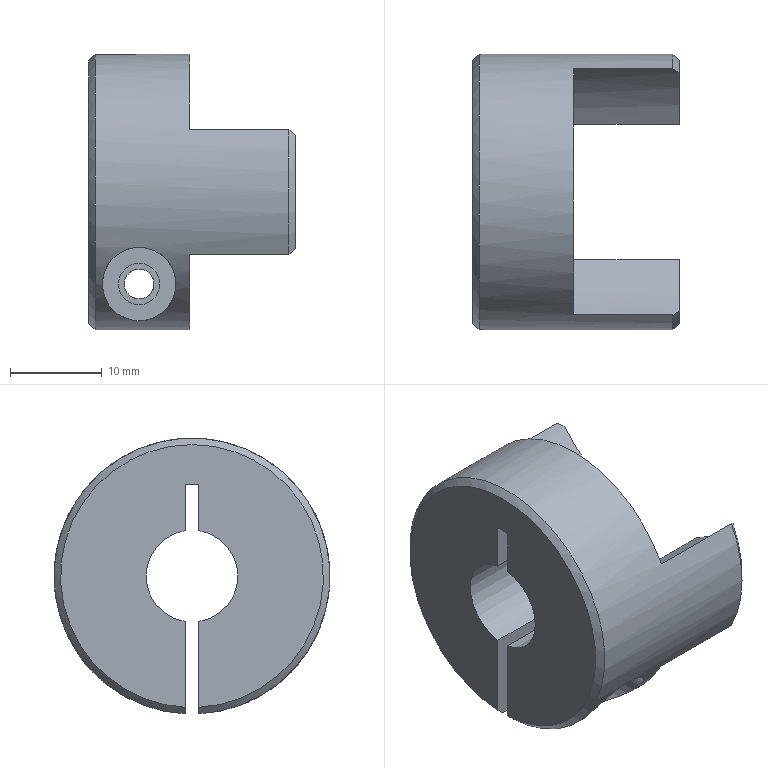Part | NX | features BREP 1 | 1 solid | 28 faces | box 22.5 x 30 x 29.981 mm | volume 7513 mm3 | cylinder 15 | plane 10 | cone 3 | commonest cylinder face diameters 32.5 x4 3.242 x2 4.5 x2 8 x2 10 x2 15 x2
STEP:
#1=CARTESIAN_POINT('',(5.5,12.442,-8.379));
#2=VERTEX_POINT('',#1);
#3=CARTESIAN_POINT('',(5.5,9.484,-11.621));
#4=VERTEX_POINT('',#3);
#5=CARTESIAN_POINT('',(5.5,12.442,-8.379));
#6=CARTESIAN_POINT('',(4.991,12.442,-8.379));
#7=CARTESIAN_POINT('',(4.064,12.098,-8.901));
#8=CARTESIAN_POINT('',(3.766,11.117,-10.112));
#9=CARTESIAN_POINT('',(4.158,10.073,-11.142));
#10=CARTESIAN_POINT('',(4.99,9.484,-11.621));
#11=CARTESIAN_POINT('',(5.5,9.484,-11.621));
#12=B_SPLINE_CURVE_WITH_KNOTS('',3,(#5,#6,#7,#8,#9,#10,#11),.UNSPECIFIED.,.F.,.F.,(4,1,1,1,4),(0.,0.001503,0.003005,0.004508,0.006011),.UNSPECIFIED.);
#13=EDGE_CURVE('',#2,#4,#12,.T.);
#14=ORIENTED_EDGE('',*,*,#13,.F.);
#15=CARTESIAN_POINT('',(5.5,0.75,-8.379));
#16=VERTEX_POINT('',#15);
#17=CARTESIAN_POINT('',(5.5,50.,-8.379));
#18=DIRECTION('',(0.,-1.,0.));
#19=VECTOR('',#18,1000.);
#20=LINE('',#17,#19);
#21=EDGE_CURVE('',#16,#2,#20,.F.);
#22=ORIENTED_EDGE('',*,*,#21,.F.);
#23=CARTESIAN_POINT('',(5.5,0.75,-11.621));
#24=VERTEX_POINT('',#23);
#25=CARTESIAN_POINT('',(5.5,0.75,-10.));
#26=DIRECTION('',(0.,1.,0.));
#27=DIRECTION('',(0.,0.,-1.));
#28=AXIS2_PLACEMENT_3D('',#25,#26,#27);
#29=CIRCLE('',#28,1.621);
#30=EDGE_CURVE('',#24,#16,#29,.T.);
#31=ORIENTED_EDGE('',*,*,#30,.F.);
#32=CARTESIAN_POINT('',(5.5,50.,-11.621));
#33=DIRECTION('',(0.,-1.,0.));
#34=VECTOR('',#33,1000.);
#35=LINE('',#32,#34);
#36=EDGE_CURVE('',#24,#4,#35,.F.);
#37=ORIENTED_EDGE('',*,*,#36,.T.);
#38=EDGE_LOOP('',(#14,#22,#31,#37));
#39=FACE_BOUND('',#38,.T.);
#40=CARTESIAN_POINT('',(5.5,50.,-10.));
#41=DIRECTION('',(0.,-1.,0.));
#42=DIRECTION('',(0.,0.,1.));
#43=AXIS2_PLACEMENT_3D('',#40,#41,#42);
#44=CYLINDRICAL_SURFACE('',#43,1.621);
#45=ADVANCED_FACE('',(#39),#44,.F.);
#46=CARTESIAN_POINT('',(5.5,-4.,-6.));
#47=VERTEX_POINT('',#46);
#48=CARTESIAN_POINT('',(5.5,-4.,-14.));
#49=VERTEX_POINT('',#48);
#50=CARTESIAN_POINT('',(5.5,-4.,-10.));
#51=DIRECTION('',(0.,-1.,0.));
#52=DIRECTION('',(0.,0.,-1.));
#53=AXIS2_PLACEMENT_3D('',#50,#51,#52);
#54=CIRCLE('',#53,4.);
#55=EDGE_CURVE('',#47,#49,#54,.T.);
#56=ORIENTED_EDGE('',*,*,#55,.F.);
#57=CARTESIAN_POINT('',(5.5,-13.748,-6.));
#58=VERTEX_POINT('',#57);
#59=CARTESIAN_POINT('',(5.5,50.,-6.));
#60=DIRECTION('',(0.,-1.,0.));
#61=VECTOR('',#60,1000.);
#62=LINE('',#59,#61);
#63=EDGE_CURVE('',#47,#58,#62,.T.);
#64=ORIENTED_EDGE('',*,*,#63,.T.);
#65=CARTESIAN_POINT('',(5.5,-5.385,-14.));
#66=VERTEX_POINT('',#65);
#67=CARTESIAN_POINT('',(5.5,-5.385,-14.));
#68=CARTESIAN_POINT('',(4.835,-5.385,-14.));
#69=CARTESIAN_POINT('',(3.735,-6.212,-13.683));
#70=CARTESIAN_POINT('',(2.69,-7.662,-12.934));
#71=CARTESIAN_POINT('',(1.917,-9.162,-11.923));
#72=CARTESIAN_POINT('',(1.333,-11.064,-10.283));
#73=CARTESIAN_POINT('',(1.701,-13.162,-7.484));
#74=CARTESIAN_POINT('',(4.177,-13.748,-6.));
#75=CARTESIAN_POINT('',(5.5,-13.748,-6.));
#76=B_SPLINE_CURVE_WITH_KNOTS('',3,(#67,#68,#69,#70,#71,#72,#73,#74,#75),.UNSPECIFIED.,.F.,.F.,(4,1,1,1,1,1,4),(0.,0.001957,0.003915,0.005872,0.00783,0.01174,0.01566),.UNSPECIFIED.);
#77=EDGE_CURVE('',#66,#58,#76,.T.);
#78=ORIENTED_EDGE('',*,*,#77,.F.);
#79=CARTESIAN_POINT('',(5.5,50.,-14.));
#80=DIRECTION('',(0.,-1.,0.));
#81=VECTOR('',#80,1000.);
#82=LINE('',#79,#81);
#83=EDGE_CURVE('',#49,#66,#82,.T.);
#84=ORIENTED_EDGE('',*,*,#83,.F.);
#85=EDGE_LOOP('',(#56,#64,#78,#84));
#86=FACE_BOUND('',#85,.T.);
#87=CARTESIAN_POINT('',(5.5,50.,-10.));
#88=DIRECTION('',(0.,-1.,0.));
#89=DIRECTION('',(0.,0.,1.));
#90=AXIS2_PLACEMENT_3D('',#87,#88,#89);
#91=CYLINDRICAL_SURFACE('',#90,4.);
#92=ADVANCED_FACE('',(#86),#91,.F.);
#93=CARTESIAN_POINT('',(5.5,-0.75,-7.75));
#94=VERTEX_POINT('',#93);
#95=CARTESIAN_POINT('',(5.5,-0.75,-12.25));
#96=VERTEX_POINT('',#95);
#97=CARTESIAN_POINT('',(5.5,-0.75,-10.));
#98=DIRECTION('',(0.,-1.,0.));
#99=DIRECTION('',(0.,0.,-1.));
#100=AXIS2_PLACEMENT_3D('',#97,#98,#99);
#101=CIRCLE('',#100,2.25);
#102=EDGE_CURVE('',#94,#96,#101,.T.);
#103=ORIENTED_EDGE('',*,*,#102,.F.);
#104=CARTESIAN_POINT('',(5.5,-4.,-7.75));
#105=VERTEX_POINT('',#104);
#106=CARTESIAN_POINT('',(5.5,50.,-7.75));
#107=DIRECTION('',(0.,-1.,0.));
#108=VECTOR('',#107,1000.);
#109=LINE('',#106,#108);
#110=EDGE_CURVE('',#105,#94,#109,.F.);
#111=ORIENTED_EDGE('',*,*,#110,.F.);
#112=CARTESIAN_POINT('',(5.5,-4.,-12.25));
#113=VERTEX_POINT('',#112);
#114=CARTESIAN_POINT('',(5.5,-4.,-10.));
#115=DIRECTION('',(0.,1.,0.));
#116=DIRECTION('',(0.,0.,-1.));
#117=AXIS2_PLACEMENT_3D('',#114,#115,#116);
#118=CIRCLE('',#117,2.25);
#119=EDGE_CURVE('',#113,#105,#118,.T.);
#120=ORIENTED_EDGE('',*,*,#119,.F.);
#121=CARTESIAN_POINT('',(5.5,50.,-12.25));
#122=DIRECTION('',(0.,-1.,0.));
#123=VECTOR('',#122,1000.);
#124=LINE('',#121,#123);
#125=EDGE_CURVE('',#113,#96,#124,.F.);
#126=ORIENTED_EDGE('',*,*,#125,.T.);
#127=EDGE_LOOP('',(#103,#111,#120,#126));
#128=FACE_BOUND('',#127,.T.);
#129=CARTESIAN_POINT('',(5.5,50.,-10.));
#130=DIRECTION('',(0.,-1.,0.));
#131=DIRECTION('',(0.,0.,1.));
#132=AXIS2_PLACEMENT_3D('',#129,#130,#131);
#133=CYLINDRICAL_SURFACE('',#132,2.25);
#134=ADVANCED_FACE('',(#128),#133,.F.);
#135=CARTESIAN_POINT('',(5.5,9.484,-11.621));
#136=CARTESIAN_POINT('',(6.011,9.484,-11.621));
#137=CARTESIAN_POINT('',(6.84,10.071,-11.144));
#138=CARTESIAN_POINT('',(7.234,11.118,-10.111));
#139=CARTESIAN_POINT('',(6.936,12.098,-8.902));
#140=CARTESIAN_POINT('',(6.009,12.442,-8.379));
#141=CARTESIAN_POINT('',(5.5,12.442,-8.379));
#142=B_SPLINE_CURVE_WITH_KNOTS('',3,(#135,#136,#137,#138,#139,#140,#141),.UNSPECIFIED.,.F.,.F.,(4,1,1,1,4),(0.,0.001502,0.003004,0.004506,0.006008),.UNSPECIFIED.);
#143=EDGE_CURVE('',#4,#2,#142,.T.);
#144=ORIENTED_EDGE('',*,*,#143,.T.);
#145=ORIENTED_EDGE('',*,*,#13,.T.);
#146=EDGE_LOOP('',(#144,#145));
#147=FACE_BOUND('',#146,.T.);
#148=CARTESIAN_POINT('',(0.7071,-0.75,-14.981));
#149=VERTEX_POINT('',#148);
#150=CARTESIAN_POINT('',(11.,-0.75,-14.981));
#151=VERTEX_POINT('',#150);
#152=CARTESIAN_POINT('',(0.,-0.75,-14.981));
#153=DIRECTION('',(1.,0.,0.));
#154=VECTOR('',#153,1000.);
#155=LINE('',#152,#154);
#156=EDGE_CURVE('',#149,#151,#155,.T.);
#157=ORIENTED_EDGE('',*,*,#156,.T.);
#158=CARTESIAN_POINT('',(11.,-13.381,-6.779));
#159=VERTEX_POINT('',#158);
#160=CARTESIAN_POINT('',(11.,0.,0.));
#161=DIRECTION('',(-1.,0.,0.));
#162=DIRECTION('',(0.,0.,-1.));
#163=AXIS2_PLACEMENT_3D('',#160,#161,#162);
#164=CIRCLE('',#163,15.);
#165=EDGE_CURVE('',#151,#159,#164,.T.);
#166=ORIENTED_EDGE('',*,*,#165,.T.);
#167=CARTESIAN_POINT('',(21.793,-13.381,-6.779));
#168=VERTEX_POINT('',#167);
#169=CARTESIAN_POINT('',(0.,-13.381,-6.779));
#170=DIRECTION('',(1.,0.,0.));
#171=VECTOR('',#170,1000.);
#172=LINE('',#169,#171);
#173=EDGE_CURVE('',#159,#168,#172,.T.);
#174=ORIENTED_EDGE('',*,*,#173,.T.);
#175=CARTESIAN_POINT('',(21.793,-13.381,6.779));
#176=VERTEX_POINT('',#175);
#177=CARTESIAN_POINT('',(21.793,0.,0.));
#178=DIRECTION('',(-1.,0.,0.));
#179=DIRECTION('',(0.,0.,-1.));
#180=AXIS2_PLACEMENT_3D('',#177,#178,#179);
#181=CIRCLE('',#180,15.);
#182=EDGE_CURVE('',#168,#176,#181,.T.);
#183=ORIENTED_EDGE('',*,*,#182,.T.);
#184=CARTESIAN_POINT('',(11.,-13.381,6.779));
#185=VERTEX_POINT('',#184);
#186=CARTESIAN_POINT('',(0.,-13.381,6.779));
#187=DIRECTION('',(-1.,0.,0.));
#188=VECTOR('',#187,1000.);
#189=LINE('',#186,#188);
#190=EDGE_CURVE('',#176,#185,#189,.T.);
#191=ORIENTED_EDGE('',*,*,#190,.T.);
#192=CARTESIAN_POINT('',(11.,13.381,6.779));
#193=VERTEX_POINT('',#192);
#194=CARTESIAN_POINT('',(11.,0.,0.));
#195=DIRECTION('',(-1.,0.,0.));
#196=DIRECTION('',(0.,0.,-1.));
#197=AXIS2_PLACEMENT_3D('',#194,#195,#196);
#198=CIRCLE('',#197,15.);
#199=EDGE_CURVE('',#185,#193,#198,.T.);
#200=ORIENTED_EDGE('',*,*,#199,.T.);
#201=CARTESIAN_POINT('',(21.793,13.381,6.779));
#202=VERTEX_POINT('',#201);
#203=CARTESIAN_POINT('',(0.,13.381,6.779));
#204=DIRECTION('',(1.,0.,0.));
#205=VECTOR('',#204,1000.);
#206=LINE('',#203,#205);
#207=EDGE_CURVE('',#193,#202,#206,.T.);
#208=ORIENTED_EDGE('',*,*,#207,.T.);
#209=CARTESIAN_POINT('',(21.793,13.381,-6.779));
#210=VERTEX_POINT('',#209);
#211=CARTESIAN_POINT('',(21.793,0.,0.));
#212=DIRECTION('',(-1.,0.,0.));
#213=DIRECTION('',(0.,0.,-1.));
#214=AXIS2_PLACEMENT_3D('',#211,#212,#213);
#215=CIRCLE('',#214,15.);
#216=EDGE_CURVE('',#202,#210,#215,.T.);
#217=ORIENTED_EDGE('',*,*,#216,.T.);
#218=CARTESIAN_POINT('',(11.,13.381,-6.779));
#219=VERTEX_POINT('',#218);
#220=CARTESIAN_POINT('',(0.,13.381,-6.779));
#221=DIRECTION('',(-1.,0.,0.));
#222=VECTOR('',#221,1000.);
#223=LINE('',#220,#222);
#224=EDGE_CURVE('',#210,#219,#223,.T.);
#225=ORIENTED_EDGE('',*,*,#224,.T.);
#226=CARTESIAN_POINT('',(11.,0.75,-14.981));
#227=VERTEX_POINT('',#226);
#228=CARTESIAN_POINT('',(11.,0.,0.));
#229=DIRECTION('',(-1.,0.,0.));
#230=DIRECTION('',(0.,0.,-1.));
#231=AXIS2_PLACEMENT_3D('',#228,#229,#230);
#232=CIRCLE('',#231,15.);
#233=EDGE_CURVE('',#219,#227,#232,.T.);
#234=ORIENTED_EDGE('',*,*,#233,.T.);
#235=CARTESIAN_POINT('',(0.7071,0.75,-14.981));
#236=VERTEX_POINT('',#235);
#237=CARTESIAN_POINT('',(0.,0.75,-14.981));
#238=DIRECTION('',(-1.,0.,0.));
#239=VECTOR('',#238,1000.);
#240=LINE('',#237,#239);
#241=EDGE_CURVE('',#227,#236,#240,.T.);
#242=ORIENTED_EDGE('',*,*,#241,.T.);
#243=CARTESIAN_POINT('',(0.7071,0.,0.));
#244=DIRECTION('',(1.,0.,0.));
#245=DIRECTION('',(0.,0.,-1.));
#246=AXIS2_PLACEMENT_3D('',#243,#244,#245);
#247=CIRCLE('',#246,15.);
#248=EDGE_CURVE('',#236,#149,#247,.T.);
#249=ORIENTED_EDGE('',*,*,#248,.T.);
#250=EDGE_LOOP('',(#157,#166,#174,#183,#191,#200,#208,#217,#225,#234,#242,#249));
#251=FACE_BOUND('',#250,.T.);
#252=ORIENTED_EDGE('',*,*,#77,.T.);
#253=CARTESIAN_POINT('',(5.5,-13.748,-6.));
#254=CARTESIAN_POINT('',(6.819,-13.748,-6.));
#255=CARTESIAN_POINT('',(8.672,-13.314,-7.082));
#256=CARTESIAN_POINT('',(9.52,-11.906,-9.196));
#257=CARTESIAN_POINT('',(9.524,-10.6,-10.673));
#258=CARTESIAN_POINT('',(9.08,-9.153,-11.932));
#259=CARTESIAN_POINT('',(8.314,-7.669,-12.929));
#260=CARTESIAN_POINT('',(7.262,-6.207,-13.686));
#261=CARTESIAN_POINT('',(6.162,-5.385,-14.));
#262=CARTESIAN_POINT('',(5.5,-5.385,-14.));
#263=B_SPLINE_CURVE_WITH_KNOTS('',3,(#253,#254,#255,#256,#257,#258,#259,#260,#261,#262),.UNSPECIFIED.,.F.,.F.,(4,1,1,1,1,1,1,4),(0.,0.003899,0.005849,0.007799,0.009748,0.0117,0.01365,0.0156),.UNSPECIFIED.);
#264=EDGE_CURVE('',#58,#66,#263,.T.);
#265=ORIENTED_EDGE('',*,*,#264,.T.);
#266=EDGE_LOOP('',(#252,#265));
#267=FACE_BOUND('',#266,.T.);
#268=CARTESIAN_POINT('',(0.,0.,0.));
#269=DIRECTION('',(1.,0.,0.));
#270=DIRECTION('',(0.,0.,1.));
#271=AXIS2_PLACEMENT_3D('',#268,#269,#270);
#272=CYLINDRICAL_SURFACE('',#271,15.);
#273=ADVANCED_FACE('',(#147,#251,#267),#272,.T.);
#274=ORIENTED_EDGE('',*,*,#21,.T.);
#275=ORIENTED_EDGE('',*,*,#143,.F.);
#276=ORIENTED_EDGE('',*,*,#36,.F.);
#277=CARTESIAN_POINT('',(5.5,0.75,-10.));
#278=DIRECTION('',(0.,1.,0.));
#279=DIRECTION('',(0.,0.,-1.));
#280=AXIS2_PLACEMENT_3D('',#277,#278,#279);
#281=CIRCLE('',#280,1.621);
#282=EDGE_CURVE('',#16,#24,#281,.T.);
#283=ORIENTED_EDGE('',*,*,#282,.F.);
#284=EDGE_LOOP('',(#274,#275,#276,#283));
#285=FACE_BOUND('',#284,.T.);
#286=CARTESIAN_POINT('',(5.5,50.,-10.));
#287=DIRECTION('',(0.,-1.,0.));
#288=DIRECTION('',(0.,0.,1.));
#289=AXIS2_PLACEMENT_3D('',#286,#287,#288);
#290=CYLINDRICAL_SURFACE('',#289,1.621);
#291=ADVANCED_FACE('',(#285),#290,.F.);
#292=CARTESIAN_POINT('',(11.,0.75,10.));
#293=VERTEX_POINT('',#292);
#294=CARTESIAN_POINT('',(11.,0.75,4.943));
#295=VERTEX_POINT('',#294);
#296=CARTESIAN_POINT('',(11.,0.75,8.));
#297=DIRECTION('',(0.,0.,-1.));
#298=VECTOR('',#297,1000.);
#299=LINE('',#296,#298);
#300=EDGE_CURVE('',#293,#295,#299,.T.);
#301=ORIENTED_EDGE('',*,*,#300,.T.);
#302=CARTESIAN_POINT('',(11.,0.75,-4.943));
#303=VERTEX_POINT('',#302);
#304=CARTESIAN_POINT('',(11.,0.,0.));
#305=DIRECTION('',(-1.,0.,0.));
#306=DIRECTION('',(0.,0.,-1.));
#307=AXIS2_PLACEMENT_3D('',#304,#305,#306);
#308=CIRCLE('',#307,5.);
#309=EDGE_CURVE('',#295,#303,#308,.T.);
#310=ORIENTED_EDGE('',*,*,#309,.T.);
#311=CARTESIAN_POINT('',(11.,0.75,8.));
#312=DIRECTION('',(0.,0.,-1.));
#313=VECTOR('',#312,1000.);
#314=LINE('',#311,#313);
#315=EDGE_CURVE('',#303,#227,#314,.T.);
#316=ORIENTED_EDGE('',*,*,#315,.T.);
#317=ORIENTED_EDGE('',*,*,#233,.F.);
#318=CARTESIAN_POINT('',(11.,7.347,-1.506));
#319=VERTEX_POINT('',#318);
#320=CARTESIAN_POINT('',(11.,0.,-16.));
#321=DIRECTION('',(1.,0.,0.));
#322=DIRECTION('',(0.,0.,-1.));
#323=AXIS2_PLACEMENT_3D('',#320,#321,#322);
#324=CIRCLE('',#323,16.25);
#325=EDGE_CURVE('',#219,#319,#324,.T.);
#326=ORIENTED_EDGE('',*,*,#325,.T.);
#327=CARTESIAN_POINT('',(11.,7.347,1.506));
#328=VERTEX_POINT('',#327);
#329=CARTESIAN_POINT('',(11.,0.,0.));
#330=DIRECTION('',(1.,0.,0.));
#331=DIRECTION('',(0.,0.,-1.));
#332=AXIS2_PLACEMENT_3D('',#329,#330,#331);
#333=CIRCLE('',#332,7.5);
#334=EDGE_CURVE('',#319,#328,#333,.T.);
#335=ORIENTED_EDGE('',*,*,#334,.T.);
#336=CARTESIAN_POINT('',(11.,0.,16.));
#337=DIRECTION('',(1.,0.,0.));
#338=DIRECTION('',(0.,0.,-1.));
#339=AXIS2_PLACEMENT_3D('',#336,#337,#338);
#340=CIRCLE('',#339,16.25);
#341=EDGE_CURVE('',#328,#193,#340,.T.);
#342=ORIENTED_EDGE('',*,*,#341,.T.);
#343=ORIENTED_EDGE('',*,*,#199,.F.);
#344=CARTESIAN_POINT('',(11.,-7.347,1.506));
#345=VERTEX_POINT('',#344);
#346=CARTESIAN_POINT('',(11.,0.,16.));
#347=DIRECTION('',(1.,0.,0.));
#348=DIRECTION('',(0.,0.,-1.));
#349=AXIS2_PLACEMENT_3D('',#346,#347,#348);
#350=CIRCLE('',#349,16.25);
#351=EDGE_CURVE('',#185,#345,#350,.T.);
#352=ORIENTED_EDGE('',*,*,#351,.T.);
#353=CARTESIAN_POINT('',(11.,-7.347,-1.506));
#354=VERTEX_POINT('',#353);
#355=CARTESIAN_POINT('',(11.,0.,0.));
#356=DIRECTION('',(1.,0.,0.));
#357=DIRECTION('',(0.,0.,-1.));
#358=AXIS2_PLACEMENT_3D('',#355,#356,#357);
#359=CIRCLE('',#358,7.5);
#360=EDGE_CURVE('',#345,#354,#359,.T.);
#361=ORIENTED_EDGE('',*,*,#360,.T.);
#362=CARTESIAN_POINT('',(11.,0.,-16.));
#363=DIRECTION('',(1.,0.,0.));
#364=DIRECTION('',(0.,0.,-1.));
#365=AXIS2_PLACEMENT_3D('',#362,#363,#364);
#366=CIRCLE('',#365,16.25);
#367=EDGE_CURVE('',#354,#159,#366,.T.);
#368=ORIENTED_EDGE('',*,*,#367,.T.);
#369=ORIENTED_EDGE('',*,*,#165,.F.);
#370=CARTESIAN_POINT('',(11.,-0.75,-4.943));
#371=VERTEX_POINT('',#370);
#372=CARTESIAN_POINT('',(11.,-0.75,8.));
#373=DIRECTION('',(0.,0.,1.));
#374=VECTOR('',#373,1000.);
#375=LINE('',#372,#374);
#376=EDGE_CURVE('',#151,#371,#375,.T.);
#377=ORIENTED_EDGE('',*,*,#376,.T.);
#378=CARTESIAN_POINT('',(11.,-0.75,4.943));
#379=VERTEX_POINT('',#378);
#380=CARTESIAN_POINT('',(11.,0.,0.));
#381=DIRECTION('',(-1.,0.,0.));
#382=DIRECTION('',(0.,0.,-1.));
#383=AXIS2_PLACEMENT_3D('',#380,#381,#382);
#384=CIRCLE('',#383,5.);
#385=EDGE_CURVE('',#371,#379,#384,.T.);
#386=ORIENTED_EDGE('',*,*,#385,.T.);
#387=CARTESIAN_POINT('',(11.,-0.75,10.));
#388=VERTEX_POINT('',#387);
#389=CARTESIAN_POINT('',(11.,-0.75,8.));
#390=DIRECTION('',(0.,0.,1.));
#391=VECTOR('',#390,1000.);
#392=LINE('',#389,#391);
#393=EDGE_CURVE('',#379,#388,#392,.T.);
#394=ORIENTED_EDGE('',*,*,#393,.T.);
#395=CARTESIAN_POINT('',(11.,0.75,10.));
#396=DIRECTION('',(0.,-1.,0.));
#397=VECTOR('',#396,1000.);
#398=LINE('',#395,#397);
#399=EDGE_CURVE('',#293,#388,#398,.T.);
#400=ORIENTED_EDGE('',*,*,#399,.F.);
#401=EDGE_LOOP('',(#301,#310,#316,#317,#326,#335,#342,#343,#352,#361,#368,#369,#377,#386,#394,#400));
#402=FACE_BOUND('',#401,.T.);
#403=CARTESIAN_POINT('',(11.,0.,8.));
#404=DIRECTION('',(1.,0.,0.));
#405=DIRECTION('',(0.,0.,1.));
#406=AXIS2_PLACEMENT_3D('',#403,#404,#405);
#407=PLANE('',#406);
#408=ADVANCED_FACE('',(#402),#407,.T.);
#409=CARTESIAN_POINT('',(0.,-0.75,-4.943));
#410=VERTEX_POINT('',#409);
#411=CARTESIAN_POINT('',(11.,-0.75,-4.943));
#412=DIRECTION('',(1.,0.,0.));
#413=VECTOR('',#412,1000.);
#414=LINE('',#411,#413);
#415=EDGE_CURVE('',#410,#371,#414,.T.);
#416=ORIENTED_EDGE('',*,*,#415,.T.);
#417=ORIENTED_EDGE('',*,*,#376,.F.);
#418=ORIENTED_EDGE('',*,*,#156,.F.);
#419=CARTESIAN_POINT('',(0.,-0.75,-14.273));
#420=VERTEX_POINT('',#419);
#421=CARTESIAN_POINT('',(0.7071,-0.75,-14.981));
#422=CARTESIAN_POINT('',(0.4714,-0.75,-14.745));
#423=CARTESIAN_POINT('',(0.2357,-0.75,-14.509));
#424=CARTESIAN_POINT('',(0.,-0.75,-14.273));
#425=B_SPLINE_CURVE_WITH_KNOTS('',3,(#421,#422,#423,#424),.UNSPECIFIED.,.F.,.F.,(4,4),(0.,1.),.PIECEWISE_BEZIER_KNOTS.);
#426=EDGE_CURVE('',#149,#420,#425,.T.);
#427=ORIENTED_EDGE('',*,*,#426,.T.);
#428=CARTESIAN_POINT('',(0.,-0.75,10.));
#429=DIRECTION('',(0.,0.,1.));
#430=VECTOR('',#429,1000.);
#431=LINE('',#428,#430);
#432=EDGE_CURVE('',#420,#410,#431,.T.);
#433=ORIENTED_EDGE('',*,*,#432,.T.);
#434=EDGE_LOOP('',(#416,#417,#418,#427,#433));
#435=FACE_BOUND('',#434,.T.);
#436=CARTESIAN_POINT('',(5.5,-0.75,-10.));
#437=DIRECTION('',(0.,-1.,0.));
#438=DIRECTION('',(0.,0.,-1.));
#439=AXIS2_PLACEMENT_3D('',#436,#437,#438);
#440=CIRCLE('',#439,2.25);
#441=EDGE_CURVE('',#96,#94,#440,.T.);
#442=ORIENTED_EDGE('',*,*,#441,.T.);
#443=ORIENTED_EDGE('',*,*,#102,.T.);
#444=EDGE_LOOP('',(#442,#443));
#445=FACE_BOUND('',#444,.T.);
#446=CARTESIAN_POINT('',(11.,-0.75,10.));
#447=DIRECTION('',(0.,1.,0.));
#448=DIRECTION('',(0.,0.,-1.));
#449=AXIS2_PLACEMENT_3D('',#446,#447,#448);
#450=PLANE('',#449);
#451=ADVANCED_FACE('',(#435,#445),#450,.T.);
#452=ORIENTED_EDGE('',*,*,#426,.F.);
#453=ORIENTED_EDGE('',*,*,#248,.F.);
#454=CARTESIAN_POINT('',(0.,0.75,-14.273));
#455=VERTEX_POINT('',#454);
#456=CARTESIAN_POINT('',(0.7071,0.75,-14.981));
#457=CARTESIAN_POINT('',(0.4714,0.75,-14.745));
#458=CARTESIAN_POINT('',(0.2357,0.75,-14.509));
#459=CARTESIAN_POINT('',(0.,0.75,-14.273));
#460=B_SPLINE_CURVE_WITH_KNOTS('',3,(#456,#457,#458,#459),.UNSPECIFIED.,.F.,.F.,(4,4),(0.,1.),.PIECEWISE_BEZIER_KNOTS.);
#461=EDGE_CURVE('',#236,#455,#460,.T.);
#462=ORIENTED_EDGE('',*,*,#461,.T.);
#463=CARTESIAN_POINT('',(0.,0.,0.));
#464=DIRECTION('',(1.,0.,0.));
#465=DIRECTION('',(0.,0.,-1.));
#466=AXIS2_PLACEMENT_3D('',#463,#464,#465);
#467=CIRCLE('',#466,14.293);
#468=EDGE_CURVE('',#455,#420,#467,.T.);
#469=ORIENTED_EDGE('',*,*,#468,.T.);
#470=EDGE_LOOP('',(#452,#453,#462,#469));
#471=FACE_BOUND('',#470,.T.);
#472=CARTESIAN_POINT('',(0.7071,0.,0.));
#473=DIRECTION('',(1.,0.,0.));
#474=DIRECTION('',(0.,0.,1.));
#475=AXIS2_PLACEMENT_3D('',#472,#473,#474);
#476=CONICAL_SURFACE('',#475,15.,0.7854);
#477=ADVANCED_FACE('',(#471),#476,.T.);
#478=CARTESIAN_POINT('',(0.,0.75,-4.943));
#479=VERTEX_POINT('',#478);
#480=CARTESIAN_POINT('',(0.,0.75,-15.));
#481=DIRECTION('',(0.,0.,-1.));
#482=VECTOR('',#481,1000.);
#483=LINE('',#480,#482);
#484=EDGE_CURVE('',#479,#455,#483,.T.);
#485=ORIENTED_EDGE('',*,*,#484,.T.);
#486=ORIENTED_EDGE('',*,*,#461,.F.);
#487=ORIENTED_EDGE('',*,*,#241,.F.);
#488=ORIENTED_EDGE('',*,*,#315,.F.);
#489=CARTESIAN_POINT('',(11.,0.75,-4.943));
#490=DIRECTION('',(-1.,0.,0.));
#491=VECTOR('',#490,1000.);
#492=LINE('',#489,#491);
#493=EDGE_CURVE('',#303,#479,#492,.T.);
#494=ORIENTED_EDGE('',*,*,#493,.T.);
#495=EDGE_LOOP('',(#485,#486,#487,#488,#494));
#496=FACE_BOUND('',#495,.T.);
#497=ORIENTED_EDGE('',*,*,#30,.T.);
#498=ORIENTED_EDGE('',*,*,#282,.T.);
#499=EDGE_LOOP('',(#497,#498));
#500=FACE_BOUND('',#499,.T.);
#501=CARTESIAN_POINT('',(11.,0.75,-15.));
#502=DIRECTION('',(0.,-1.,0.));
#503=DIRECTION('',(0.,0.,1.));
#504=AXIS2_PLACEMENT_3D('',#501,#502,#503);
#505=PLANE('',#504);
#506=ADVANCED_FACE('',(#496,#500),#505,.T.);
#507=CARTESIAN_POINT('',(22.5,7.347,-1.506));
#508=VERTEX_POINT('',#507);
#509=CARTESIAN_POINT('',(46.,7.347,-1.506));
#510=DIRECTION('',(1.,0.,0.));
#511=VECTOR('',#510,1000.);
#512=LINE('',#509,#511);
#513=EDGE_CURVE('',#319,#508,#512,.T.);
#514=ORIENTED_EDGE('',*,*,#513,.F.);
#515=ORIENTED_EDGE('',*,*,#325,.F.);
#516=ORIENTED_EDGE('',*,*,#224,.F.);
#517=CARTESIAN_POINT('',(22.5,12.911,-6.132));
#518=VERTEX_POINT('',#517);
#519=CARTESIAN_POINT('',(22.5,12.911,-6.132));
#520=CARTESIAN_POINT('',(22.263,13.072,-6.343));
#521=CARTESIAN_POINT('',(22.028,13.229,-6.559));
#522=CARTESIAN_POINT('',(21.793,13.381,-6.779));
#523=B_SPLINE_CURVE_WITH_KNOTS('',3,(#519,#520,#521,#522),.UNSPECIFIED.,.F.,.F.,(4,4),(0.,1.),.PIECEWISE_BEZIER_KNOTS.);
#524=EDGE_CURVE('',#518,#210,#523,.T.);
#525=ORIENTED_EDGE('',*,*,#524,.F.);
#526=CARTESIAN_POINT('',(22.5,0.,-16.));
#527=DIRECTION('',(-1.,0.,0.));
#528=DIRECTION('',(0.,0.,-1.));
#529=AXIS2_PLACEMENT_3D('',#526,#527,#528);
#530=CIRCLE('',#529,16.25);
#531=EDGE_CURVE('',#508,#518,#530,.T.);
#532=ORIENTED_EDGE('',*,*,#531,.F.);
#533=EDGE_LOOP('',(#514,#515,#516,#525,#532));
#534=FACE_BOUND('',#533,.T.);
#535=CARTESIAN_POINT('',(46.,0.,-16.));
#536=DIRECTION('',(1.,0.,0.));
#537=DIRECTION('',(0.,0.,1.));
#538=AXIS2_PLACEMENT_3D('',#535,#536,#537);
#539=CYLINDRICAL_SURFACE('',#538,16.25);
#540=ADVANCED_FACE('',(#534),#539,.F.);
#541=ORIENTED_EDGE('',*,*,#524,.T.);
#542=ORIENTED_EDGE('',*,*,#216,.F.);
#543=CARTESIAN_POINT('',(22.5,12.911,6.132));
#544=VERTEX_POINT('',#543);
#545=CARTESIAN_POINT('',(21.793,13.381,6.779));
#546=CARTESIAN_POINT('',(22.028,13.229,6.559));
#547=CARTESIAN_POINT('',(22.263,13.072,6.343));
#548=CARTESIAN_POINT('',(22.5,12.911,6.132));
#549=B_SPLINE_CURVE_WITH_KNOTS('',3,(#545,#546,#547,#548),.UNSPECIFIED.,.F.,.F.,(4,4),(0.,1.),.PIECEWISE_BEZIER_KNOTS.);
#550=EDGE_CURVE('',#202,#544,#549,.T.);
#551=ORIENTED_EDGE('',*,*,#550,.T.);
#552=CARTESIAN_POINT('',(22.5,0.,0.));
#553=DIRECTION('',(-1.,0.,0.));
#554=DIRECTION('',(0.,0.,1.));
#555=AXIS2_PLACEMENT_3D('',#552,#553,#554);
#556=CIRCLE('',#555,14.293);
#557=EDGE_CURVE('',#544,#518,#556,.T.);
#558=ORIENTED_EDGE('',*,*,#557,.T.);
#559=EDGE_LOOP('',(#541,#542,#551,#558));
#560=FACE_BOUND('',#559,.T.);
#561=CARTESIAN_POINT('',(21.793,0.,0.));
#562=DIRECTION('',(-1.,0.,0.));
#563=DIRECTION('',(0.,0.,-1.));
#564=AXIS2_PLACEMENT_3D('',#561,#562,#563);
#565=CONICAL_SURFACE('',#564,15.,0.7854);
#566=ADVANCED_FACE('',(#560),#565,.T.);
#567=ORIENTED_EDGE('',*,*,#550,.F.);
#568=ORIENTED_EDGE('',*,*,#207,.F.);
#569=ORIENTED_EDGE('',*,*,#341,.F.);
#570=CARTESIAN_POINT('',(22.5,7.347,1.506));
#571=VERTEX_POINT('',#570);
#572=CARTESIAN_POINT('',(46.,7.347,1.506));
#573=DIRECTION('',(-1.,0.,0.));
#574=VECTOR('',#573,1000.);
#575=LINE('',#572,#574);
#576=EDGE_CURVE('',#571,#328,#575,.T.);
#577=ORIENTED_EDGE('',*,*,#576,.F.);
#578=CARTESIAN_POINT('',(22.5,0.,16.));
#579=DIRECTION('',(-1.,0.,0.));
#580=DIRECTION('',(0.,0.,-1.));
#581=AXIS2_PLACEMENT_3D('',#578,#579,#580);
#582=CIRCLE('',#581,16.25);
#583=EDGE_CURVE('',#544,#571,#582,.T.);
#584=ORIENTED_EDGE('',*,*,#583,.F.);
#585=EDGE_LOOP('',(#567,#568,#569,#577,#584));
#586=FACE_BOUND('',#585,.T.);
#587=CARTESIAN_POINT('',(46.,0.,16.));
#588=DIRECTION('',(1.,0.,0.));
#589=DIRECTION('',(0.,0.,1.));
#590=AXIS2_PLACEMENT_3D('',#587,#588,#589);
#591=CYLINDRICAL_SURFACE('',#590,16.25);
#592=ADVANCED_FACE('',(#586),#591,.F.);
#593=CARTESIAN_POINT('',(22.5,-7.347,1.506));
#594=VERTEX_POINT('',#593);
#595=CARTESIAN_POINT('',(46.,-7.347,1.506));
#596=DIRECTION('',(1.,0.,0.));
#597=VECTOR('',#596,1000.);
#598=LINE('',#595,#597);
#599=EDGE_CURVE('',#345,#594,#598,.T.);
#600=ORIENTED_EDGE('',*,*,#599,.F.);
#601=ORIENTED_EDGE('',*,*,#351,.F.);
#602=ORIENTED_EDGE('',*,*,#190,.F.);
#603=CARTESIAN_POINT('',(22.5,-12.911,6.132));
#604=VERTEX_POINT('',#603);
#605=CARTESIAN_POINT('',(22.5,-12.911,6.132));
#606=CARTESIAN_POINT('',(22.263,-13.072,6.343));
#607=CARTESIAN_POINT('',(22.028,-13.229,6.559));
#608=CARTESIAN_POINT('',(21.793,-13.381,6.779));
#609=B_SPLINE_CURVE_WITH_KNOTS('',3,(#605,#606,#607,#608),.UNSPECIFIED.,.F.,.F.,(4,4),(0.,1.),.PIECEWISE_BEZIER_KNOTS.);
#610=EDGE_CURVE('',#604,#176,#609,.T.);
#611=ORIENTED_EDGE('',*,*,#610,.F.);
#612=CARTESIAN_POINT('',(22.5,0.,16.));
#613=DIRECTION('',(-1.,0.,0.));
#614=DIRECTION('',(0.,0.,-1.));
#615=AXIS2_PLACEMENT_3D('',#612,#613,#614);
#616=CIRCLE('',#615,16.25);
#617=EDGE_CURVE('',#594,#604,#616,.T.);
#618=ORIENTED_EDGE('',*,*,#617,.F.);
#619=EDGE_LOOP('',(#600,#601,#602,#611,#618));
#620=FACE_BOUND('',#619,.T.);
#621=CARTESIAN_POINT('',(46.,0.,16.));
#622=DIRECTION('',(1.,0.,0.));
#623=DIRECTION('',(0.,0.,1.));
#624=AXIS2_PLACEMENT_3D('',#621,#622,#623);
#625=CYLINDRICAL_SURFACE('',#624,16.25);
#626=ADVANCED_FACE('',(#620),#625,.F.);
#627=ORIENTED_EDGE('',*,*,#610,.T.);
#628=ORIENTED_EDGE('',*,*,#182,.F.);
#629=CARTESIAN_POINT('',(22.5,-12.911,-6.132));
#630=VERTEX_POINT('',#629);
#631=CARTESIAN_POINT('',(21.793,-13.381,-6.779));
#632=CARTESIAN_POINT('',(22.028,-13.229,-6.559));
#633=CARTESIAN_POINT('',(22.263,-13.072,-6.343));
#634=CARTESIAN_POINT('',(22.5,-12.911,-6.132));
#635=B_SPLINE_CURVE_WITH_KNOTS('',3,(#631,#632,#633,#634),.UNSPECIFIED.,.F.,.F.,(4,4),(0.,1.),.PIECEWISE_BEZIER_KNOTS.);
#636=EDGE_CURVE('',#168,#630,#635,.T.);
#637=ORIENTED_EDGE('',*,*,#636,.T.);
#638=CARTESIAN_POINT('',(22.5,0.,0.));
#639=DIRECTION('',(-1.,0.,0.));
#640=DIRECTION('',(0.,0.,1.));
#641=AXIS2_PLACEMENT_3D('',#638,#639,#640);
#642=CIRCLE('',#641,14.293);
#643=EDGE_CURVE('',#630,#604,#642,.T.);
#644=ORIENTED_EDGE('',*,*,#643,.T.);
#645=EDGE_LOOP('',(#627,#628,#637,#644));
#646=FACE_BOUND('',#645,.T.);
#647=CARTESIAN_POINT('',(21.793,0.,0.));
#648=DIRECTION('',(-1.,0.,0.));
#649=DIRECTION('',(0.,0.,-1.));
#650=AXIS2_PLACEMENT_3D('',#647,#648,#649);
#651=CONICAL_SURFACE('',#650,15.,0.7854);
#652=ADVANCED_FACE('',(#646),#651,.T.);
#653=ORIENTED_EDGE('',*,*,#636,.F.);
#654=ORIENTED_EDGE('',*,*,#173,.F.);
#655=ORIENTED_EDGE('',*,*,#367,.F.);
#656=CARTESIAN_POINT('',(22.5,-7.347,-1.506));
#657=VERTEX_POINT('',#656);
#658=CARTESIAN_POINT('',(46.,-7.347,-1.506));
#659=DIRECTION('',(-1.,0.,0.));
#660=VECTOR('',#659,1000.);
#661=LINE('',#658,#660);
#662=EDGE_CURVE('',#657,#354,#661,.T.);
#663=ORIENTED_EDGE('',*,*,#662,.F.);
#664=CARTESIAN_POINT('',(22.5,0.,-16.));
#665=DIRECTION('',(-1.,0.,0.));
#666=DIRECTION('',(0.,0.,-1.));
#667=AXIS2_PLACEMENT_3D('',#664,#665,#666);
#668=CIRCLE('',#667,16.25);
#669=EDGE_CURVE('',#630,#657,#668,.T.);
#670=ORIENTED_EDGE('',*,*,#669,.F.);
#671=EDGE_LOOP('',(#653,#654,#655,#663,#670));
#672=FACE_BOUND('',#671,.T.);
#673=CARTESIAN_POINT('',(46.,0.,-16.));
#674=DIRECTION('',(1.,0.,0.));
#675=DIRECTION('',(0.,0.,1.));
#676=AXIS2_PLACEMENT_3D('',#673,#674,#675);
#677=CYLINDRICAL_SURFACE('',#676,16.25);
#678=ADVANCED_FACE('',(#672),#677,.F.);
#679=ORIENTED_EDGE('',*,*,#63,.F.);
#680=CARTESIAN_POINT('',(5.5,-4.,-10.));
#681=DIRECTION('',(0.,-1.,0.));
#682=DIRECTION('',(0.,0.,-1.));
#683=AXIS2_PLACEMENT_3D('',#680,#681,#682);
#684=CIRCLE('',#683,4.);
#685=EDGE_CURVE('',#49,#47,#684,.T.);
#686=ORIENTED_EDGE('',*,*,#685,.F.);
#687=ORIENTED_EDGE('',*,*,#83,.T.);
#688=ORIENTED_EDGE('',*,*,#264,.F.);
#689=EDGE_LOOP('',(#679,#686,#687,#688));
#690=FACE_BOUND('',#689,.T.);
#691=CARTESIAN_POINT('',(5.5,50.,-10.));
#692=DIRECTION('',(0.,-1.,0.));
#693=DIRECTION('',(0.,0.,1.));
#694=AXIS2_PLACEMENT_3D('',#691,#692,#693);
#695=CYLINDRICAL_SURFACE('',#694,4.);
#696=ADVANCED_FACE('',(#690),#695,.F.);
#697=ORIENTED_EDGE('',*,*,#309,.F.);
#698=CARTESIAN_POINT('',(0.,0.75,4.943));
#699=VERTEX_POINT('',#698);
#700=CARTESIAN_POINT('',(35.,0.75,4.943));
#701=DIRECTION('',(1.,0.,0.));
#702=VECTOR('',#701,1000.);
#703=LINE('',#700,#702);
#704=EDGE_CURVE('',#699,#295,#703,.T.);
#705=ORIENTED_EDGE('',*,*,#704,.F.);
#706=CARTESIAN_POINT('',(0.,0.,0.));
#707=DIRECTION('',(1.,0.,0.));
#708=DIRECTION('',(0.,0.,-1.));
#709=AXIS2_PLACEMENT_3D('',#706,#707,#708);
#710=CIRCLE('',#709,5.);
#711=EDGE_CURVE('',#479,#699,#710,.T.);
#712=ORIENTED_EDGE('',*,*,#711,.F.);
#713=ORIENTED_EDGE('',*,*,#493,.F.);
#714=EDGE_LOOP('',(#697,#705,#712,#713));
#715=FACE_BOUND('',#714,.T.);
#716=CARTESIAN_POINT('',(35.,0.,0.));
#717=DIRECTION('',(1.,0.,0.));
#718=DIRECTION('',(0.,0.,1.));
#719=AXIS2_PLACEMENT_3D('',#716,#717,#718);
#720=CYLINDRICAL_SURFACE('',#719,5.);
#721=ADVANCED_FACE('',(#715),#720,.F.);
#722=CARTESIAN_POINT('',(0.,0.75,10.));
#723=VERTEX_POINT('',#722);
#724=CARTESIAN_POINT('',(0.,0.75,-15.));
#725=DIRECTION('',(0.,0.,-1.));
#726=VECTOR('',#725,1000.);
#727=LINE('',#724,#726);
#728=EDGE_CURVE('',#723,#699,#727,.T.);
#729=ORIENTED_EDGE('',*,*,#728,.T.);
#730=ORIENTED_EDGE('',*,*,#704,.T.);
#731=ORIENTED_EDGE('',*,*,#300,.F.);
#732=CARTESIAN_POINT('',(11.,0.75,10.));
#733=DIRECTION('',(-1.,0.,0.));
#734=VECTOR('',#733,1000.);
#735=LINE('',#732,#734);
#736=EDGE_CURVE('',#293,#723,#735,.T.);
#737=ORIENTED_EDGE('',*,*,#736,.T.);
#738=EDGE_LOOP('',(#729,#730,#731,#737));
#739=FACE_BOUND('',#738,.T.);
#740=CARTESIAN_POINT('',(11.,0.75,-15.));
#741=DIRECTION('',(0.,-1.,0.));
#742=DIRECTION('',(0.,0.,1.));
#743=AXIS2_PLACEMENT_3D('',#740,#741,#742);
#744=PLANE('',#743);
#745=ADVANCED_FACE('',(#739),#744,.T.);
#746=ORIENTED_EDGE('',*,*,#393,.F.);
#747=CARTESIAN_POINT('',(0.,-0.75,4.943));
#748=VERTEX_POINT('',#747);
#749=CARTESIAN_POINT('',(11.,-0.75,4.943));
#750=DIRECTION('',(-1.,0.,0.));
#751=VECTOR('',#750,1000.);
#752=LINE('',#749,#751);
#753=EDGE_CURVE('',#379,#748,#752,.T.);
#754=ORIENTED_EDGE('',*,*,#753,.T.);
#755=CARTESIAN_POINT('',(0.,-0.75,10.));
#756=VERTEX_POINT('',#755);
#757=CARTESIAN_POINT('',(0.,-0.75,10.));
#758=DIRECTION('',(0.,0.,1.));
#759=VECTOR('',#758,1000.);
#760=LINE('',#757,#759);
#761=EDGE_CURVE('',#748,#756,#760,.T.);
#762=ORIENTED_EDGE('',*,*,#761,.T.);
#763=CARTESIAN_POINT('',(11.,-0.75,10.));
#764=DIRECTION('',(1.,0.,0.));
#765=VECTOR('',#764,1000.);
#766=LINE('',#763,#765);
#767=EDGE_CURVE('',#756,#388,#766,.T.);
#768=ORIENTED_EDGE('',*,*,#767,.T.);
#769=EDGE_LOOP('',(#746,#754,#762,#768));
#770=FACE_BOUND('',#769,.T.);
#771=CARTESIAN_POINT('',(11.,-0.75,10.));
#772=DIRECTION('',(0.,1.,0.));
#773=DIRECTION('',(0.,0.,-1.));
#774=AXIS2_PLACEMENT_3D('',#771,#772,#773);
#775=PLANE('',#774);
#776=ADVANCED_FACE('',(#770),#775,.T.);
#777=ORIENTED_EDGE('',*,*,#385,.F.);
#778=ORIENTED_EDGE('',*,*,#415,.F.);
#779=CARTESIAN_POINT('',(0.,0.,0.));
#780=DIRECTION('',(1.,0.,0.));
#781=DIRECTION('',(0.,0.,-1.));
#782=AXIS2_PLACEMENT_3D('',#779,#780,#781);
#783=CIRCLE('',#782,5.);
#784=EDGE_CURVE('',#748,#410,#783,.T.);
#785=ORIENTED_EDGE('',*,*,#784,.F.);
#786=ORIENTED_EDGE('',*,*,#753,.F.);
#787=EDGE_LOOP('',(#777,#778,#785,#786));
#788=FACE_BOUND('',#787,.T.);
#789=CARTESIAN_POINT('',(35.,0.,0.));
#790=DIRECTION('',(1.,0.,0.));
#791=DIRECTION('',(0.,0.,1.));
#792=AXIS2_PLACEMENT_3D('',#789,#790,#791);
#793=CYLINDRICAL_SURFACE('',#792,5.);
#794=ADVANCED_FACE('',(#788),#793,.F.);
#795=CARTESIAN_POINT('',(22.5,0.,0.));
#796=DIRECTION('',(-1.,0.,0.));
#797=DIRECTION('',(0.,0.,-1.));
#798=AXIS2_PLACEMENT_3D('',#795,#796,#797);
#799=CIRCLE('',#798,7.5);
#800=EDGE_CURVE('',#657,#594,#799,.T.);
#801=ORIENTED_EDGE('',*,*,#800,.F.);
#802=ORIENTED_EDGE('',*,*,#662,.T.);
#803=ORIENTED_EDGE('',*,*,#360,.F.);
#804=ORIENTED_EDGE('',*,*,#599,.T.);
#805=EDGE_LOOP('',(#801,#802,#803,#804));
#806=FACE_BOUND('',#805,.T.);
#807=CARTESIAN_POINT('',(46.,0.,0.));
#808=DIRECTION('',(1.,0.,0.));
#809=DIRECTION('',(0.,0.,1.));
#810=AXIS2_PLACEMENT_3D('',#807,#808,#809);
#811=CYLINDRICAL_SURFACE('',#810,7.5);
#812=ADVANCED_FACE('',(#806),#811,.F.);
#813=ORIENTED_EDGE('',*,*,#576,.T.);
#814=ORIENTED_EDGE('',*,*,#334,.F.);
#815=ORIENTED_EDGE('',*,*,#513,.T.);
#816=CARTESIAN_POINT('',(22.5,0.,0.));
#817=DIRECTION('',(-1.,0.,0.));
#818=DIRECTION('',(0.,0.,-1.));
#819=AXIS2_PLACEMENT_3D('',#816,#817,#818);
#820=CIRCLE('',#819,7.5);
#821=EDGE_CURVE('',#571,#508,#820,.T.);
#822=ORIENTED_EDGE('',*,*,#821,.F.);
#823=EDGE_LOOP('',(#813,#814,#815,#822));
#824=FACE_BOUND('',#823,.T.);
#825=CARTESIAN_POINT('',(46.,0.,0.));
#826=DIRECTION('',(1.,0.,0.));
#827=DIRECTION('',(0.,0.,1.));
#828=AXIS2_PLACEMENT_3D('',#825,#826,#827);
#829=CYLINDRICAL_SURFACE('',#828,7.5);
#830=ADVANCED_FACE('',(#824),#829,.F.);
#831=ORIENTED_EDGE('',*,*,#784,.T.);
#832=ORIENTED_EDGE('',*,*,#432,.F.);
#833=ORIENTED_EDGE('',*,*,#468,.F.);
#834=ORIENTED_EDGE('',*,*,#484,.F.);
#835=ORIENTED_EDGE('',*,*,#711,.T.);
#836=ORIENTED_EDGE('',*,*,#728,.F.);
#837=CARTESIAN_POINT('',(0.,-14.293,10.));
#838=DIRECTION('',(0.,1.,0.));
#839=VECTOR('',#838,1000.);
#840=LINE('',#837,#839);
#841=EDGE_CURVE('',#756,#723,#840,.T.);
#842=ORIENTED_EDGE('',*,*,#841,.F.);
#843=ORIENTED_EDGE('',*,*,#761,.F.);
#844=EDGE_LOOP('',(#831,#832,#833,#834,#835,#836,#842,#843));
#845=FACE_BOUND('',#844,.T.);
#846=CARTESIAN_POINT('',(0.,-14.293,0.));
#847=DIRECTION('',(1.,0.,0.));
#848=DIRECTION('',(0.,0.,1.));
#849=AXIS2_PLACEMENT_3D('',#846,#847,#848);
#850=PLANE('',#849);
#851=ADVANCED_FACE('',(#845),#850,.F.);
#852=ORIENTED_EDGE('',*,*,#110,.T.);
#853=ORIENTED_EDGE('',*,*,#441,.F.);
#854=ORIENTED_EDGE('',*,*,#125,.F.);
#855=CARTESIAN_POINT('',(5.5,-4.,-10.));
#856=DIRECTION('',(0.,1.,0.));
#857=DIRECTION('',(0.,0.,-1.));
#858=AXIS2_PLACEMENT_3D('',#855,#856,#857);
#859=CIRCLE('',#858,2.25);
#860=EDGE_CURVE('',#105,#113,#859,.T.);
#861=ORIENTED_EDGE('',*,*,#860,.F.);
#862=EDGE_LOOP('',(#852,#853,#854,#861));
#863=FACE_BOUND('',#862,.T.);
#864=CARTESIAN_POINT('',(5.5,50.,-10.));
#865=DIRECTION('',(0.,-1.,0.));
#866=DIRECTION('',(0.,0.,1.));
#867=AXIS2_PLACEMENT_3D('',#864,#865,#866);
#868=CYLINDRICAL_SURFACE('',#867,2.25);
#869=ADVANCED_FACE('',(#863),#868,.F.);
#870=ORIENTED_EDGE('',*,*,#821,.T.);
#871=ORIENTED_EDGE('',*,*,#531,.T.);
#872=ORIENTED_EDGE('',*,*,#557,.F.);
#873=ORIENTED_EDGE('',*,*,#583,.T.);
#874=EDGE_LOOP('',(#870,#871,#872,#873));
#875=FACE_BOUND('',#874,.T.);
#876=CARTESIAN_POINT('',(22.5,0.,0.));
#877=DIRECTION('',(-1.,0.,0.));
#878=DIRECTION('',(0.,0.,-1.));
#879=AXIS2_PLACEMENT_3D('',#876,#877,#878);
#880=PLANE('',#879);
#881=ADVANCED_FACE('',(#875),#880,.F.);
#882=ORIENTED_EDGE('',*,*,#617,.T.);
#883=ORIENTED_EDGE('',*,*,#643,.F.);
#884=ORIENTED_EDGE('',*,*,#669,.T.);
#885=ORIENTED_EDGE('',*,*,#800,.T.);
#886=EDGE_LOOP('',(#882,#883,#884,#885));
#887=FACE_BOUND('',#886,.T.);
#888=CARTESIAN_POINT('',(22.5,0.,0.));
#889=DIRECTION('',(-1.,0.,0.));
#890=DIRECTION('',(0.,0.,-1.));
#891=AXIS2_PLACEMENT_3D('',#888,#889,#890);
#892=PLANE('',#891);
#893=ADVANCED_FACE('',(#887),#892,.F.);
#894=ORIENTED_EDGE('',*,*,#685,.T.);
#895=ORIENTED_EDGE('',*,*,#55,.T.);
#896=EDGE_LOOP('',(#894,#895));
#897=FACE_BOUND('',#896,.T.);
#898=ORIENTED_EDGE('',*,*,#119,.T.);
#899=ORIENTED_EDGE('',*,*,#860,.T.);
#900=EDGE_LOOP('',(#898,#899));
#901=FACE_BOUND('',#900,.T.);
#902=CARTESIAN_POINT('',(5.5,-4.,-6.));
#903=DIRECTION('',(0.,-1.,0.));
#904=DIRECTION('',(0.,0.,1.));
#905=AXIS2_PLACEMENT_3D('',#902,#903,#904);
#906=PLANE('',#905);
#907=ADVANCED_FACE('',(#897,#901),#906,.T.);
#908=ORIENTED_EDGE('',*,*,#399,.T.);
#909=ORIENTED_EDGE('',*,*,#767,.F.);
#910=ORIENTED_EDGE('',*,*,#841,.T.);
#911=ORIENTED_EDGE('',*,*,#736,.F.);
#912=EDGE_LOOP('',(#908,#909,#910,#911));
#913=FACE_BOUND('',#912,.T.);
#914=CARTESIAN_POINT('',(11.,0.75,10.));
#915=DIRECTION('',(0.,0.,-1.));
#916=DIRECTION('',(1.,0.,0.));
#917=AXIS2_PLACEMENT_3D('',#914,#915,#916);
#918=PLANE('',#917);
#919=ADVANCED_FACE('',(#913),#918,.T.);
#920=CLOSED_SHELL('',(#45,#92,#134,#273,#291,#408,#451,#477,#506,#540,#566,#592,#626,#652,#678,#696,#721,#745,#776,#794,#812,#830,#851,#869,#881,#893,#907,#919));
#921=MANIFOLD_SOLID_BREP('',#920);
#922=(LENGTH_UNIT()NAMED_UNIT(*)SI_UNIT(.MILLI.,.METRE.));
#923=UNCERTAINTY_MEASURE_WITH_UNIT(LENGTH_MEASURE(0.0508),#922,'','');
#924=(NAMED_UNIT(*)PLANE_ANGLE_UNIT()SI_UNIT($,.RADIAN.));
#925=(NAMED_UNIT(*)SI_UNIT($,.STERADIAN.)SOLID_ANGLE_UNIT());
#926=(GEOMETRIC_REPRESENTATION_CONTEXT(3)GLOBAL_UNCERTAINTY_ASSIGNED_CONTEXT((#923))GLOBAL_UNIT_ASSIGNED_CONTEXT((#922,#924,#925))REPRESENTATION_CONTEXT('',''));
#927=ADVANCED_BREP_SHAPE_REPRESENTATION('',(#921),#926);